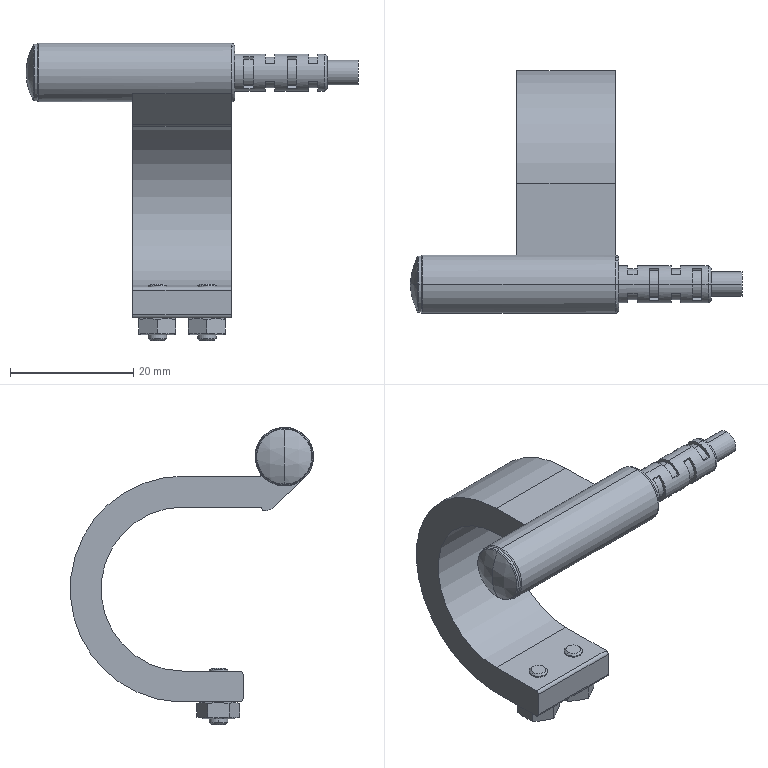Part | STEP file | CS1_B6 | 1 solid | 136 faces | box 53.8 x 39.45 x 48.2 mm | volume 8992 mm3 | plane 77 | cylinder 33 | cone 16 | torus 8 | sphere 2 | commonest cylinder face diameters 5 x10 3 x9 1 x2 4 x2 6 x2 9.2 x2